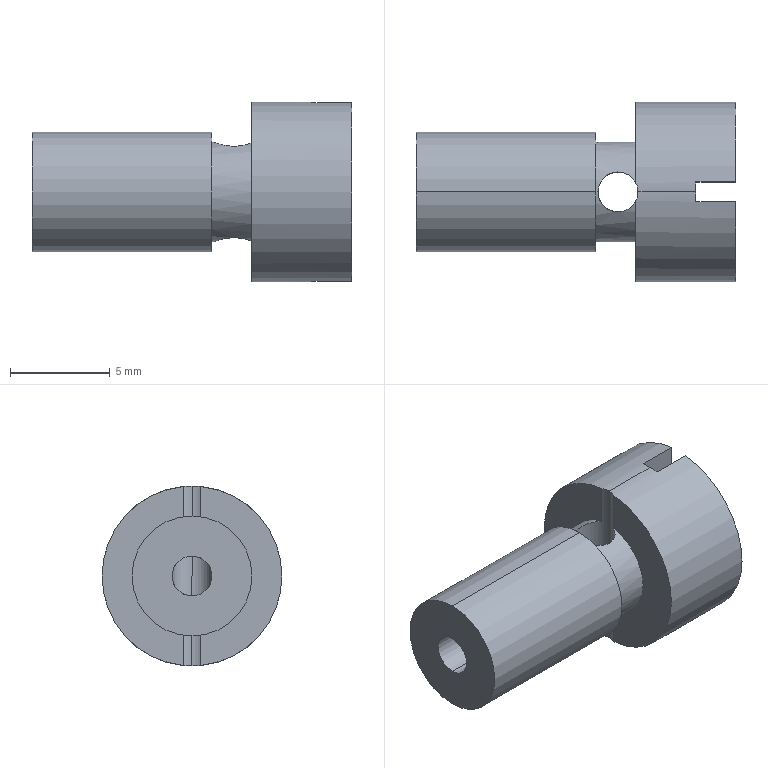Part | SolidWorks | features ICE 5, Extrusion 1 | 1 solid | 19 faces | box 16 x 9 x 9 mm | volume 549.177 mm3 | cylinder 10 | plane 9 | commonest cylinder face diameters 2 x4 5 x2 6 x2 9 x2
STEP:
#1=CARTESIAN_POINT('',(9.1,0.,-2.5));
#2=VERTEX_POINT('',#1);
#3=CARTESIAN_POINT('',(11.,-0.4359,-2.462));
#4=VERTEX_POINT('',#3);
#5=CARTESIAN_POINT('',(9.1,0.,-2.5));
#6=CARTESIAN_POINT('',(9.1,-0.1141,-2.5));
#7=CARTESIAN_POINT('',(9.119,-0.2264,-2.492));
#8=CARTESIAN_POINT('',(9.195,-0.4393,-2.463));
#9=CARTESIAN_POINT('',(9.25,-0.538,-2.443));
#10=CARTESIAN_POINT('',(9.458,-0.7984,-2.376));
#11=CARTESIAN_POINT('',(9.655,-0.9237,-2.324));
#12=CARTESIAN_POINT('',(9.985,-0.9998,-2.292));
#13=CARTESIAN_POINT('',(10.1,-1.006,-2.289));
#14=CARTESIAN_POINT('',(10.325,-0.9809,-2.3));
#15=CARTESIAN_POINT('',(10.435,-0.9488,-2.314));
#16=CARTESIAN_POINT('',(10.737,-0.8027,-2.37));
#17=CARTESIAN_POINT('',(10.901,-0.6393,-2.426));
#18=CARTESIAN_POINT('',(11.,-0.4359,-2.462));
#19=B_SPLINE_CURVE_WITH_KNOTS('',3,(#5,#6,#7,#8,#9,#10,#11,#12,#13,#14,#15,#16,#17,#18),.UNSPECIFIED.,.F.,.F.,(4,2,2,2,2,2,4),(0.002708,0.003047,0.003385,0.004061,0.004399,0.004738,0.005414),.UNSPECIFIED.);
#20=EDGE_CURVE('',#2,#4,#19,.T.);
#21=ORIENTED_EDGE('',*,*,#20,.F.);
#22=CARTESIAN_POINT('',(9.1,0.,-1.));
#23=VERTEX_POINT('',#22);
#24=CARTESIAN_POINT('',(9.1,0.,-4.5));
#25=DIRECTION('',(0.,0.,1.));
#26=VECTOR('',#25,1000.);
#27=LINE('',#24,#26);
#28=EDGE_CURVE('',#2,#23,#27,.T.);
#29=ORIENTED_EDGE('',*,*,#28,.T.);
#30=CARTESIAN_POINT('',(10.1,-1.,0.));
#31=VERTEX_POINT('',#30);
#32=CARTESIAN_POINT('',(9.1,0.,-1.));
#33=CARTESIAN_POINT('',(9.1,-0.5858,-1.));
#34=CARTESIAN_POINT('',(9.514,-1.,-0.5858));
#35=CARTESIAN_POINT('',(10.1,-1.,0.));
#36=(BOUNDED_CURVE()B_SPLINE_CURVE(3,(#32,#33,#34,#35),.UNSPECIFIED.,.F.,.T.)B_SPLINE_CURVE_WITH_KNOTS((4,4),(3.142,4.712),.UNSPECIFIED.)CURVE()GEOMETRIC_REPRESENTATION_ITEM()RATIONAL_B_SPLINE_CURVE((1.,0.8047,0.8047,1.))REPRESENTATION_ITEM(''));
#37=EDGE_CURVE('',#23,#31,#36,.T.);
#38=ORIENTED_EDGE('',*,*,#37,.T.);
#39=CARTESIAN_POINT('',(9.1,0.,1.));
#40=VERTEX_POINT('',#39);
#41=CARTESIAN_POINT('',(10.1,-1.,0.));
#42=CARTESIAN_POINT('',(9.514,-1.,0.5858));
#43=CARTESIAN_POINT('',(9.1,-0.5858,1.));
#44=CARTESIAN_POINT('',(9.1,0.,1.));
#45=(BOUNDED_CURVE()B_SPLINE_CURVE(3,(#41,#42,#43,#44),.UNSPECIFIED.,.F.,.F.)B_SPLINE_CURVE_WITH_KNOTS((4,4),(1.571,3.142),.UNSPECIFIED.)CURVE()GEOMETRIC_REPRESENTATION_ITEM()RATIONAL_B_SPLINE_CURVE((1.,0.8047,0.8047,1.))REPRESENTATION_ITEM(''));
#46=EDGE_CURVE('',#31,#40,#45,.T.);
#47=ORIENTED_EDGE('',*,*,#46,.T.);
#48=CARTESIAN_POINT('',(9.1,0.,2.5));
#49=VERTEX_POINT('',#48);
#50=CARTESIAN_POINT('',(9.1,0.,-4.5));
#51=DIRECTION('',(0.,0.,1.));
#52=VECTOR('',#51,1000.);
#53=LINE('',#50,#52);
#54=EDGE_CURVE('',#40,#49,#53,.T.);
#55=ORIENTED_EDGE('',*,*,#54,.T.);
#56=CARTESIAN_POINT('',(11.,-0.4359,2.462));
#57=VERTEX_POINT('',#56);
#58=CARTESIAN_POINT('',(11.,-0.4359,2.462));
#59=CARTESIAN_POINT('',(10.901,-0.6395,2.426));
#60=CARTESIAN_POINT('',(10.739,-0.8012,2.37));
#61=CARTESIAN_POINT('',(10.435,-0.9488,2.314));
#62=CARTESIAN_POINT('',(10.328,-0.9804,2.3));
#63=CARTESIAN_POINT('',(10.101,-1.006,2.288));
#64=CARTESIAN_POINT('',(9.987,-1.,2.291));
#65=CARTESIAN_POINT('',(9.654,-0.9237,2.324));
#66=CARTESIAN_POINT('',(9.458,-0.7988,2.376));
#67=CARTESIAN_POINT('',(9.179,-0.45,2.466));
#68=CARTESIAN_POINT('',(9.1,-0.2283,2.5));
#69=CARTESIAN_POINT('',(9.1,0.,2.5));
#70=B_SPLINE_CURVE_WITH_KNOTS('',3,(#58,#59,#60,#61,#62,#63,#64,#65,#66,#67,#68,#69),.UNSPECIFIED.,.F.,.F.,(4,2,2,2,2,4),(0.,0.0006771,0.001016,0.001354,0.002031,0.002708),.UNSPECIFIED.);
#71=EDGE_CURVE('',#57,#49,#70,.T.);
#72=ORIENTED_EDGE('',*,*,#71,.F.);
#73=CARTESIAN_POINT('',(11.,-0.4359,4.479));
#74=VERTEX_POINT('',#73);
#75=CARTESIAN_POINT('',(11.,-0.4359,-4.5));
#76=DIRECTION('',(0.,0.,-1.));
#77=VECTOR('',#76,1000.);
#78=LINE('',#75,#77);
#79=EDGE_CURVE('',#74,#57,#78,.T.);
#80=ORIENTED_EDGE('',*,*,#79,.F.);
#81=CARTESIAN_POINT('',(11.1,0.,4.5));
#82=VERTEX_POINT('',#81);
#83=CARTESIAN_POINT('',(11.1,0.,4.5));
#84=CARTESIAN_POINT('',(11.1,-0.1517,4.5));
#85=CARTESIAN_POINT('',(11.066,-0.2999,4.492));
#86=CARTESIAN_POINT('',(11.,-0.4359,4.479));
#87=B_SPLINE_CURVE_WITH_KNOTS('',3,(#83,#84,#85,#86),.UNSPECIFIED.,.F.,.F.,(4,4),(0.0004486,0.0008971),.UNSPECIFIED.);
#88=EDGE_CURVE('',#82,#74,#87,.T.);
#89=ORIENTED_EDGE('',*,*,#88,.F.);
#90=CARTESIAN_POINT('',(11.1,0.,-4.5));
#91=VERTEX_POINT('',#90);
#92=CARTESIAN_POINT('',(11.1,0.,-4.5));
#93=DIRECTION('',(0.,0.,1.));
#94=VECTOR('',#93,1000.);
#95=LINE('',#92,#94);
#96=EDGE_CURVE('',#91,#82,#95,.T.);
#97=ORIENTED_EDGE('',*,*,#96,.F.);
#98=CARTESIAN_POINT('',(11.,-0.4359,-4.479));
#99=VERTEX_POINT('',#98);
#100=CARTESIAN_POINT('',(11.,-0.4359,-4.479));
#101=CARTESIAN_POINT('',(11.066,-0.2999,-4.492));
#102=CARTESIAN_POINT('',(11.1,-0.1517,-4.5));
#103=CARTESIAN_POINT('',(11.1,0.,-4.5));
#104=B_SPLINE_CURVE_WITH_KNOTS('',3,(#100,#101,#102,#103),.UNSPECIFIED.,.F.,.F.,(4,4),(0.,0.0004486),.UNSPECIFIED.);
#105=EDGE_CURVE('',#99,#91,#104,.T.);
#106=ORIENTED_EDGE('',*,*,#105,.F.);
#107=CARTESIAN_POINT('',(11.,-0.4359,-4.5));
#108=DIRECTION('',(0.,0.,-1.));
#109=VECTOR('',#108,1000.);
#110=LINE('',#107,#109);
#111=EDGE_CURVE('',#4,#99,#110,.T.);
#112=ORIENTED_EDGE('',*,*,#111,.F.);
#113=EDGE_LOOP('',(#21,#29,#38,#47,#55,#72,#80,#89,#97,#106,#112));
#114=FACE_OUTER_BOUND('',#113,.T.);
#115=CARTESIAN_POINT('',(10.1,0.,-4.5));
#116=DIRECTION('',(0.,0.,1.));
#117=DIRECTION('',(1.,0.,0.));
#118=AXIS2_PLACEMENT_3D('',#115,#116,#117);
#119=CYLINDRICAL_SURFACE('',#118,1.);
#120=ADVANCED_FACE('',(#114),#119,.F.);
#121=CARTESIAN_POINT('',(0.,0.,-1.));
#122=VERTEX_POINT('',#121);
#123=CARTESIAN_POINT('',(0.,0.,1.));
#124=VERTEX_POINT('',#123);
#125=CARTESIAN_POINT('',(0.,0.,0.));
#126=DIRECTION('',(-1.,0.,0.));
#127=DIRECTION('',(0.,0.,-1.));
#128=AXIS2_PLACEMENT_3D('',#125,#126,#127);
#129=CIRCLE('',#128,1.);
#130=EDGE_CURVE('',#122,#124,#129,.T.);
#131=ORIENTED_EDGE('',*,*,#130,.T.);
#132=CARTESIAN_POINT('',(-0.000012,0.,1.));
#133=DIRECTION('',(1.,0.,0.));
#134=VECTOR('',#133,1000.);
#135=LINE('',#132,#134);
#136=EDGE_CURVE('',#124,#40,#135,.T.);
#137=ORIENTED_EDGE('',*,*,#136,.T.);
#138=ORIENTED_EDGE('',*,*,#46,.F.);
#139=ORIENTED_EDGE('',*,*,#37,.F.);
#140=CARTESIAN_POINT('',(-0.000012,0.,-1.));
#141=DIRECTION('',(1.,0.,0.));
#142=VECTOR('',#141,1000.);
#143=LINE('',#140,#142);
#144=EDGE_CURVE('',#122,#23,#143,.T.);
#145=ORIENTED_EDGE('',*,*,#144,.F.);
#146=EDGE_LOOP('',(#131,#137,#138,#139,#145));
#147=FACE_OUTER_BOUND('',#146,.T.);
#148=CARTESIAN_POINT('',(-0.000012,0.,0.));
#149=DIRECTION('',(1.,0.,0.));
#150=DIRECTION('',(0.,0.,-1.));
#151=AXIS2_PLACEMENT_3D('',#148,#149,#150);
#152=CYLINDRICAL_SURFACE('',#151,1.);
#153=ADVANCED_FACE('',(#147),#152,.F.);
#154=CARTESIAN_POINT('',(14.,0.5,-4.472));
#155=VERTEX_POINT('',#154);
#156=CARTESIAN_POINT('',(14.,0.,-4.5));
#157=VERTEX_POINT('',#156);
#158=CARTESIAN_POINT('',(14.,0.,0.));
#159=DIRECTION('',(-1.,0.,0.));
#160=DIRECTION('',(0.,-1.,0.));
#161=AXIS2_PLACEMENT_3D('',#158,#159,#160);
#162=CIRCLE('',#161,4.5);
#163=EDGE_CURVE('',#155,#157,#162,.T.);
#164=ORIENTED_EDGE('',*,*,#163,.T.);
#165=CARTESIAN_POINT('',(16.,0.,-4.5));
#166=DIRECTION('',(-1.,0.,0.));
#167=VECTOR('',#166,1000.);
#168=LINE('',#165,#167);
#169=EDGE_CURVE('',#157,#91,#168,.T.);
#170=ORIENTED_EDGE('',*,*,#169,.T.);
#171=CARTESIAN_POINT('',(11.,0.4359,-4.479));
#172=VERTEX_POINT('',#171);
#173=CARTESIAN_POINT('',(11.1,0.,-4.5));
#174=CARTESIAN_POINT('',(11.1,0.1517,-4.5));
#175=CARTESIAN_POINT('',(11.066,0.2999,-4.492));
#176=CARTESIAN_POINT('',(11.,0.4359,-4.479));
#177=B_SPLINE_CURVE_WITH_KNOTS('',3,(#173,#174,#175,#176),.UNSPECIFIED.,.F.,.F.,(4,4),(0.0004486,0.0008971),.UNSPECIFIED.);
#178=EDGE_CURVE('',#91,#172,#177,.T.);
#179=ORIENTED_EDGE('',*,*,#178,.T.);
#180=CARTESIAN_POINT('',(11.,0.4359,4.479));
#181=VERTEX_POINT('',#180);
#182=CARTESIAN_POINT('',(11.,0.,0.));
#183=DIRECTION('',(1.,0.,0.));
#184=DIRECTION('',(0.,0.,-1.));
#185=AXIS2_PLACEMENT_3D('',#182,#183,#184);
#186=CIRCLE('',#185,4.5);
#187=EDGE_CURVE('',#172,#181,#186,.T.);
#188=ORIENTED_EDGE('',*,*,#187,.T.);
#189=CARTESIAN_POINT('',(11.,0.4359,4.479));
#190=CARTESIAN_POINT('',(11.066,0.2999,4.492));
#191=CARTESIAN_POINT('',(11.1,0.1517,4.5));
#192=CARTESIAN_POINT('',(11.1,0.,4.5));
#193=B_SPLINE_CURVE_WITH_KNOTS('',3,(#189,#190,#191,#192),.UNSPECIFIED.,.F.,.F.,(4,4),(0.,0.0004486),.UNSPECIFIED.);
#194=EDGE_CURVE('',#181,#82,#193,.T.);
#195=ORIENTED_EDGE('',*,*,#194,.T.);
#196=CARTESIAN_POINT('',(14.,0.,4.5));
#197=VERTEX_POINT('',#196);
#198=CARTESIAN_POINT('',(16.,0.,4.5));
#199=DIRECTION('',(-1.,0.,0.));
#200=VECTOR('',#199,1000.);
#201=LINE('',#198,#200);
#202=EDGE_CURVE('',#197,#82,#201,.T.);
#203=ORIENTED_EDGE('',*,*,#202,.F.);
#204=CARTESIAN_POINT('',(14.,0.5,4.472));
#205=VERTEX_POINT('',#204);
#206=CARTESIAN_POINT('',(14.,0.,0.));
#207=DIRECTION('',(-1.,0.,0.));
#208=DIRECTION('',(0.,-1.,0.));
#209=AXIS2_PLACEMENT_3D('',#206,#207,#208);
#210=CIRCLE('',#209,4.5);
#211=EDGE_CURVE('',#197,#205,#210,.T.);
#212=ORIENTED_EDGE('',*,*,#211,.T.);
#213=CARTESIAN_POINT('',(16.,0.5,4.472));
#214=VERTEX_POINT('',#213);
#215=CARTESIAN_POINT('',(16.,0.5,4.472));
#216=DIRECTION('',(1.,0.,0.));
#217=VECTOR('',#216,1000.);
#218=LINE('',#215,#217);
#219=EDGE_CURVE('',#205,#214,#218,.T.);
#220=ORIENTED_EDGE('',*,*,#219,.T.);
#221=CARTESIAN_POINT('',(16.,0.5,-4.472));
#222=VERTEX_POINT('',#221);
#223=CARTESIAN_POINT('',(16.,0.,0.));
#224=DIRECTION('',(1.,0.,0.));
#225=DIRECTION('',(0.,0.,-1.));
#226=AXIS2_PLACEMENT_3D('',#223,#224,#225);
#227=CIRCLE('',#226,4.5);
#228=EDGE_CURVE('',#222,#214,#227,.T.);
#229=ORIENTED_EDGE('',*,*,#228,.F.);
#230=CARTESIAN_POINT('',(16.,0.5,-4.472));
#231=DIRECTION('',(-1.,0.,0.));
#232=VECTOR('',#231,1000.);
#233=LINE('',#230,#232);
#234=EDGE_CURVE('',#222,#155,#233,.T.);
#235=ORIENTED_EDGE('',*,*,#234,.T.);
#236=EDGE_LOOP('',(#164,#170,#179,#188,#195,#203,#212,#220,#229,#235));
#237=FACE_OUTER_BOUND('',#236,.T.);
#238=CARTESIAN_POINT('',(16.,0.,0.));
#239=DIRECTION('',(-1.,0.,0.));
#240=DIRECTION('',(0.,0.,1.));
#241=AXIS2_PLACEMENT_3D('',#238,#239,#240);
#242=CYLINDRICAL_SURFACE('',#241,4.5);
#243=ADVANCED_FACE('',(#237),#242,.T.);
#244=CARTESIAN_POINT('',(11.,0.4359,-2.462));
#245=VERTEX_POINT('',#244);
#246=CARTESIAN_POINT('',(11.,0.4359,-2.462));
#247=CARTESIAN_POINT('',(10.901,0.6395,-2.426));
#248=CARTESIAN_POINT('',(10.739,0.8012,-2.37));
#249=CARTESIAN_POINT('',(10.435,0.9488,-2.314));
#250=CARTESIAN_POINT('',(10.328,0.9804,-2.3));
#251=CARTESIAN_POINT('',(10.101,1.006,-2.288));
#252=CARTESIAN_POINT('',(9.987,1.,-2.291));
#253=CARTESIAN_POINT('',(9.654,0.9237,-2.324));
#254=CARTESIAN_POINT('',(9.458,0.7988,-2.376));
#255=CARTESIAN_POINT('',(9.179,0.45,-2.466));
#256=CARTESIAN_POINT('',(9.1,0.2283,-2.5));
#257=CARTESIAN_POINT('',(9.1,0.,-2.5));
#258=B_SPLINE_CURVE_WITH_KNOTS('',3,(#246,#247,#248,#249,#250,#251,#252,#253,#254,#255,#256,#257),.UNSPECIFIED.,.F.,.F.,(4,2,2,2,2,4),(0.,0.0006771,0.001016,0.001354,0.002031,0.002708),.UNSPECIFIED.);
#259=EDGE_CURVE('',#245,#2,#258,.T.);
#260=ORIENTED_EDGE('',*,*,#259,.T.);
#261=CARTESIAN_POINT('',(9.,0.,-2.5));
#262=VERTEX_POINT('',#261);
#263=CARTESIAN_POINT('',(11.,0.,-2.5));
#264=DIRECTION('',(-1.,0.,0.));
#265=VECTOR('',#264,1000.);
#266=LINE('',#263,#265);
#267=EDGE_CURVE('',#2,#262,#266,.T.);
#268=ORIENTED_EDGE('',*,*,#267,.T.);
#269=CARTESIAN_POINT('',(9.,0.,2.5));
#270=VERTEX_POINT('',#269);
#271=CARTESIAN_POINT('',(9.,0.,0.));
#272=DIRECTION('',(1.,0.,0.));
#273=DIRECTION('',(0.,0.,-1.));
#274=AXIS2_PLACEMENT_3D('',#271,#272,#273);
#275=CIRCLE('',#274,2.5);
#276=EDGE_CURVE('',#262,#270,#275,.T.);
#277=ORIENTED_EDGE('',*,*,#276,.T.);
#278=CARTESIAN_POINT('',(11.,0.,2.5));
#279=DIRECTION('',(-1.,0.,0.));
#280=VECTOR('',#279,1000.);
#281=LINE('',#278,#280);
#282=EDGE_CURVE('',#49,#270,#281,.T.);
#283=ORIENTED_EDGE('',*,*,#282,.F.);
#284=CARTESIAN_POINT('',(11.,0.4359,2.462));
#285=VERTEX_POINT('',#284);
#286=CARTESIAN_POINT('',(9.1,0.,2.5));
#287=CARTESIAN_POINT('',(9.1,0.1141,2.5));
#288=CARTESIAN_POINT('',(9.119,0.2264,2.492));
#289=CARTESIAN_POINT('',(9.195,0.4393,2.463));
#290=CARTESIAN_POINT('',(9.25,0.538,2.443));
#291=CARTESIAN_POINT('',(9.458,0.7984,2.376));
#292=CARTESIAN_POINT('',(9.655,0.9237,2.324));
#293=CARTESIAN_POINT('',(9.985,0.9998,2.292));
#294=CARTESIAN_POINT('',(10.1,1.006,2.289));
#295=CARTESIAN_POINT('',(10.325,0.9809,2.3));
#296=CARTESIAN_POINT('',(10.435,0.9488,2.314));
#297=CARTESIAN_POINT('',(10.737,0.8027,2.37));
#298=CARTESIAN_POINT('',(10.901,0.6393,2.426));
#299=CARTESIAN_POINT('',(11.,0.4359,2.462));
#300=B_SPLINE_CURVE_WITH_KNOTS('',3,(#286,#287,#288,#289,#290,#291,#292,#293,#294,#295,#296,#297,#298,#299),.UNSPECIFIED.,.F.,.F.,(4,2,2,2,2,2,4),(0.002708,0.003047,0.003385,0.004061,0.004399,0.004738,0.005414),.UNSPECIFIED.);
#301=EDGE_CURVE('',#49,#285,#300,.T.);
#302=ORIENTED_EDGE('',*,*,#301,.T.);
#303=CARTESIAN_POINT('',(11.,0.,0.));
#304=DIRECTION('',(1.,0.,0.));
#305=DIRECTION('',(0.,0.,-1.));
#306=AXIS2_PLACEMENT_3D('',#303,#304,#305);
#307=CIRCLE('',#306,2.5);
#308=EDGE_CURVE('',#245,#285,#307,.T.);
#309=ORIENTED_EDGE('',*,*,#308,.F.);
#310=EDGE_LOOP('',(#260,#268,#277,#283,#302,#309));
#311=FACE_OUTER_BOUND('',#310,.T.);
#312=CARTESIAN_POINT('',(11.,0.,0.));
#313=DIRECTION('',(-1.,0.,0.));
#314=DIRECTION('',(0.,0.,1.));
#315=AXIS2_PLACEMENT_3D('',#312,#313,#314);
#316=CYLINDRICAL_SURFACE('',#315,2.5);
#317=ADVANCED_FACE('',(#311),#316,.T.);
#318=CARTESIAN_POINT('',(9.,0.,-3.));
#319=VERTEX_POINT('',#318);
#320=CARTESIAN_POINT('',(9.,0.,3.));
#321=VERTEX_POINT('',#320);
#322=CARTESIAN_POINT('',(9.,0.,0.));
#323=DIRECTION('',(1.,0.,0.));
#324=DIRECTION('',(0.,0.,-1.));
#325=AXIS2_PLACEMENT_3D('',#322,#323,#324);
#326=CIRCLE('',#325,3.);
#327=EDGE_CURVE('',#319,#321,#326,.T.);
#328=ORIENTED_EDGE('',*,*,#327,.F.);
#329=CARTESIAN_POINT('',(0.,0.,-3.));
#330=VERTEX_POINT('',#329);
#331=CARTESIAN_POINT('',(9.,0.,-3.));
#332=DIRECTION('',(-1.,0.,0.));
#333=VECTOR('',#332,1000.);
#334=LINE('',#331,#333);
#335=EDGE_CURVE('',#319,#330,#334,.T.);
#336=ORIENTED_EDGE('',*,*,#335,.T.);
#337=CARTESIAN_POINT('',(0.,0.,3.));
#338=VERTEX_POINT('',#337);
#339=CARTESIAN_POINT('',(0.,0.,0.));
#340=DIRECTION('',(1.,0.,0.));
#341=DIRECTION('',(0.,0.,-1.));
#342=AXIS2_PLACEMENT_3D('',#339,#340,#341);
#343=CIRCLE('',#342,3.);
#344=EDGE_CURVE('',#330,#338,#343,.T.);
#345=ORIENTED_EDGE('',*,*,#344,.T.);
#346=CARTESIAN_POINT('',(9.,0.,3.));
#347=DIRECTION('',(-1.,0.,0.));
#348=VECTOR('',#347,1000.);
#349=LINE('',#346,#348);
#350=EDGE_CURVE('',#321,#338,#349,.T.);
#351=ORIENTED_EDGE('',*,*,#350,.F.);
#352=EDGE_LOOP('',(#328,#336,#345,#351));
#353=FACE_OUTER_BOUND('',#352,.T.);
#354=CARTESIAN_POINT('',(9.,0.,0.));
#355=DIRECTION('',(-1.,0.,0.));
#356=DIRECTION('',(0.,0.,1.));
#357=AXIS2_PLACEMENT_3D('',#354,#355,#356);
#358=CYLINDRICAL_SURFACE('',#357,3.);
#359=ADVANCED_FACE('',(#353),#358,.T.);
#360=CARTESIAN_POINT('',(16.,-0.5,4.472));
#361=VERTEX_POINT('',#360);
#362=CARTESIAN_POINT('',(16.,-0.5,-4.472));
#363=VERTEX_POINT('',#362);
#364=CARTESIAN_POINT('',(16.,-0.5,0.));
#365=DIRECTION('',(0.,0.,-1.));
#366=VECTOR('',#365,1000.);
#367=LINE('',#364,#366);
#368=EDGE_CURVE('',#361,#363,#367,.T.);
#369=ORIENTED_EDGE('',*,*,#368,.F.);
#370=CARTESIAN_POINT('',(16.,0.,0.));
#371=DIRECTION('',(1.,0.,0.));
#372=DIRECTION('',(0.,0.,-1.));
#373=AXIS2_PLACEMENT_3D('',#370,#371,#372);
#374=CIRCLE('',#373,4.5);
#375=EDGE_CURVE('',#361,#363,#374,.T.);
#376=ORIENTED_EDGE('',*,*,#375,.T.);
#377=EDGE_LOOP('',(#369,#376));
#378=FACE_OUTER_BOUND('',#377,.T.);
#379=CARTESIAN_POINT('',(16.,0.,0.));
#380=DIRECTION('',(1.,0.,0.));
#381=DIRECTION('',(0.,0.,-1.));
#382=AXIS2_PLACEMENT_3D('',#379,#380,#381);
#383=PLANE('',#382);
#384=ADVANCED_FACE('',(#378),#383,.T.);
#385=ORIENTED_EDGE('',*,*,#187,.F.);
#386=CARTESIAN_POINT('',(11.,0.4359,-4.5));
#387=DIRECTION('',(0.,0.,1.));
#388=VECTOR('',#387,1000.);
#389=LINE('',#386,#388);
#390=EDGE_CURVE('',#172,#245,#389,.T.);
#391=ORIENTED_EDGE('',*,*,#390,.T.);
#392=ORIENTED_EDGE('',*,*,#308,.T.);
#393=CARTESIAN_POINT('',(11.,0.4359,-4.5));
#394=DIRECTION('',(0.,0.,1.));
#395=VECTOR('',#394,1000.);
#396=LINE('',#393,#395);
#397=EDGE_CURVE('',#285,#181,#396,.T.);
#398=ORIENTED_EDGE('',*,*,#397,.T.);
#399=EDGE_LOOP('',(#385,#391,#392,#398));
#400=FACE_OUTER_BOUND('',#399,.T.);
#401=CARTESIAN_POINT('',(11.,0.,0.));
#402=DIRECTION('',(1.,0.,0.));
#403=DIRECTION('',(0.,0.,-1.));
#404=AXIS2_PLACEMENT_3D('',#401,#402,#403);
#405=PLANE('',#404);
#406=ADVANCED_FACE('',(#400),#405,.F.);
#407=ORIENTED_EDGE('',*,*,#335,.F.);
#408=CARTESIAN_POINT('',(9.,0.,0.));
#409=DIRECTION('',(1.,0.,0.));
#410=DIRECTION('',(0.,0.,-1.));
#411=AXIS2_PLACEMENT_3D('',#408,#409,#410);
#412=CIRCLE('',#411,3.);
#413=EDGE_CURVE('',#321,#319,#412,.T.);
#414=ORIENTED_EDGE('',*,*,#413,.F.);
#415=ORIENTED_EDGE('',*,*,#350,.T.);
#416=CARTESIAN_POINT('',(0.,0.,0.));
#417=DIRECTION('',(1.,0.,0.));
#418=DIRECTION('',(0.,0.,-1.));
#419=AXIS2_PLACEMENT_3D('',#416,#417,#418);
#420=CIRCLE('',#419,3.);
#421=EDGE_CURVE('',#338,#330,#420,.T.);
#422=ORIENTED_EDGE('',*,*,#421,.T.);
#423=EDGE_LOOP('',(#407,#414,#415,#422));
#424=FACE_OUTER_BOUND('',#423,.T.);
#425=CARTESIAN_POINT('',(9.,0.,0.));
#426=DIRECTION('',(-1.,0.,0.));
#427=DIRECTION('',(0.,0.,1.));
#428=AXIS2_PLACEMENT_3D('',#425,#426,#427);
#429=CYLINDRICAL_SURFACE('',#428,3.);
#430=ADVANCED_FACE('',(#424),#429,.T.);
#431=CARTESIAN_POINT('',(9.,0.,0.));
#432=DIRECTION('',(1.,0.,0.));
#433=DIRECTION('',(0.,0.,-1.));
#434=AXIS2_PLACEMENT_3D('',#431,#432,#433);
#435=CIRCLE('',#434,2.5);
#436=EDGE_CURVE('',#270,#262,#435,.T.);
#437=ORIENTED_EDGE('',*,*,#436,.F.);
#438=ORIENTED_EDGE('',*,*,#276,.F.);
#439=EDGE_LOOP('',(#437,#438));
#440=FACE_BOUND('',#439,.T.);
#441=ORIENTED_EDGE('',*,*,#413,.T.);
#442=ORIENTED_EDGE('',*,*,#327,.T.);
#443=EDGE_LOOP('',(#441,#442));
#444=FACE_OUTER_BOUND('',#443,.T.);
#445=CARTESIAN_POINT('',(9.,0.,0.));
#446=DIRECTION('',(1.,0.,0.));
#447=DIRECTION('',(0.,0.,-1.));
#448=AXIS2_PLACEMENT_3D('',#445,#446,#447);
#449=PLANE('',#448);
#450=ADVANCED_FACE('',(#440,#444),#449,.T.);
#451=ORIENTED_EDGE('',*,*,#130,.F.);
#452=CARTESIAN_POINT('',(0.,0.,0.));
#453=DIRECTION('',(-1.,0.,0.));
#454=DIRECTION('',(0.,0.,-1.));
#455=AXIS2_PLACEMENT_3D('',#452,#453,#454);
#456=CIRCLE('',#455,1.);
#457=EDGE_CURVE('',#124,#122,#456,.T.);
#458=ORIENTED_EDGE('',*,*,#457,.F.);
#459=EDGE_LOOP('',(#451,#458));
#460=FACE_BOUND('',#459,.T.);
#461=ORIENTED_EDGE('',*,*,#421,.F.);
#462=ORIENTED_EDGE('',*,*,#344,.F.);
#463=EDGE_LOOP('',(#461,#462));
#464=FACE_OUTER_BOUND('',#463,.T.);
#465=CARTESIAN_POINT('',(0.,0.,0.));
#466=DIRECTION('',(1.,0.,0.));
#467=DIRECTION('',(0.,0.,-1.));
#468=AXIS2_PLACEMENT_3D('',#465,#466,#467);
#469=PLANE('',#468);
#470=ADVANCED_FACE('',(#460,#464),#469,.F.);
#471=ORIENTED_EDGE('',*,*,#267,.F.);
#472=ORIENTED_EDGE('',*,*,#20,.T.);
#473=CARTESIAN_POINT('',(11.,0.,0.));
#474=DIRECTION('',(1.,0.,0.));
#475=DIRECTION('',(0.,0.,-1.));
#476=AXIS2_PLACEMENT_3D('',#473,#474,#475);
#477=CIRCLE('',#476,2.5);
#478=EDGE_CURVE('',#57,#4,#477,.T.);
#479=ORIENTED_EDGE('',*,*,#478,.F.);
#480=ORIENTED_EDGE('',*,*,#71,.T.);
#481=ORIENTED_EDGE('',*,*,#282,.T.);
#482=ORIENTED_EDGE('',*,*,#436,.T.);
#483=EDGE_LOOP('',(#471,#472,#479,#480,#481,#482));
#484=FACE_OUTER_BOUND('',#483,.T.);
#485=CARTESIAN_POINT('',(11.,0.,0.));
#486=DIRECTION('',(-1.,0.,0.));
#487=DIRECTION('',(0.,0.,1.));
#488=AXIS2_PLACEMENT_3D('',#485,#486,#487);
#489=CYLINDRICAL_SURFACE('',#488,2.5);
#490=ADVANCED_FACE('',(#484),#489,.T.);
#491=ORIENTED_EDGE('',*,*,#169,.F.);
#492=CARTESIAN_POINT('',(14.,-0.5,-4.472));
#493=VERTEX_POINT('',#492);
#494=CARTESIAN_POINT('',(14.,0.,0.));
#495=DIRECTION('',(-1.,0.,0.));
#496=DIRECTION('',(0.,-1.,0.));
#497=AXIS2_PLACEMENT_3D('',#494,#495,#496);
#498=CIRCLE('',#497,4.5);
#499=EDGE_CURVE('',#157,#493,#498,.T.);
#500=ORIENTED_EDGE('',*,*,#499,.T.);
#501=CARTESIAN_POINT('',(16.,-0.5,-4.472));
#502=DIRECTION('',(1.,0.,0.));
#503=VECTOR('',#502,1000.);
#504=LINE('',#501,#503);
#505=EDGE_CURVE('',#493,#363,#504,.T.);
#506=ORIENTED_EDGE('',*,*,#505,.T.);
#507=ORIENTED_EDGE('',*,*,#375,.F.);
#508=CARTESIAN_POINT('',(14.,-0.5,4.472));
#509=VERTEX_POINT('',#508);
#510=CARTESIAN_POINT('',(16.,-0.5,4.472));
#511=DIRECTION('',(-1.,0.,0.));
#512=VECTOR('',#511,1000.);
#513=LINE('',#510,#512);
#514=EDGE_CURVE('',#361,#509,#513,.T.);
#515=ORIENTED_EDGE('',*,*,#514,.T.);
#516=CARTESIAN_POINT('',(14.,0.,0.));
#517=DIRECTION('',(-1.,0.,0.));
#518=DIRECTION('',(0.,-1.,0.));
#519=AXIS2_PLACEMENT_3D('',#516,#517,#518);
#520=CIRCLE('',#519,4.5);
#521=EDGE_CURVE('',#509,#197,#520,.T.);
#522=ORIENTED_EDGE('',*,*,#521,.T.);
#523=ORIENTED_EDGE('',*,*,#202,.T.);
#524=ORIENTED_EDGE('',*,*,#88,.T.);
#525=CARTESIAN_POINT('',(11.,0.,0.));
#526=DIRECTION('',(1.,0.,0.));
#527=DIRECTION('',(0.,0.,-1.));
#528=AXIS2_PLACEMENT_3D('',#525,#526,#527);
#529=CIRCLE('',#528,4.5);
#530=EDGE_CURVE('',#74,#99,#529,.T.);
#531=ORIENTED_EDGE('',*,*,#530,.T.);
#532=ORIENTED_EDGE('',*,*,#105,.T.);
#533=EDGE_LOOP('',(#491,#500,#506,#507,#515,#522,#523,#524,#531,#532));
#534=FACE_OUTER_BOUND('',#533,.T.);
#535=CARTESIAN_POINT('',(16.,0.,0.));
#536=DIRECTION('',(-1.,0.,0.));
#537=DIRECTION('',(0.,0.,1.));
#538=AXIS2_PLACEMENT_3D('',#535,#536,#537);
#539=CYLINDRICAL_SURFACE('',#538,4.5);
#540=ADVANCED_FACE('',(#534),#539,.T.);
#541=CARTESIAN_POINT('',(16.,0.5,0.));
#542=DIRECTION('',(0.,0.,1.));
#543=VECTOR('',#542,1000.);
#544=LINE('',#541,#543);
#545=EDGE_CURVE('',#222,#214,#544,.T.);
#546=ORIENTED_EDGE('',*,*,#545,.F.);
#547=ORIENTED_EDGE('',*,*,#228,.T.);
#548=EDGE_LOOP('',(#546,#547));
#549=FACE_OUTER_BOUND('',#548,.T.);
#550=CARTESIAN_POINT('',(16.,0.,0.));
#551=DIRECTION('',(1.,0.,0.));
#552=DIRECTION('',(0.,0.,-1.));
#553=AXIS2_PLACEMENT_3D('',#550,#551,#552);
#554=PLANE('',#553);
#555=ADVANCED_FACE('',(#549),#554,.T.);
#556=ORIENTED_EDGE('',*,*,#530,.F.);
#557=ORIENTED_EDGE('',*,*,#79,.T.);
#558=ORIENTED_EDGE('',*,*,#478,.T.);
#559=ORIENTED_EDGE('',*,*,#111,.T.);
#560=EDGE_LOOP('',(#556,#557,#558,#559));
#561=FACE_OUTER_BOUND('',#560,.T.);
#562=CARTESIAN_POINT('',(11.,0.,0.));
#563=DIRECTION('',(1.,0.,0.));
#564=DIRECTION('',(0.,0.,-1.));
#565=AXIS2_PLACEMENT_3D('',#562,#563,#564);
#566=PLANE('',#565);
#567=ADVANCED_FACE('',(#561),#566,.F.);
#568=ORIENTED_EDGE('',*,*,#136,.F.);
#569=ORIENTED_EDGE('',*,*,#457,.T.);
#570=ORIENTED_EDGE('',*,*,#144,.T.);
#571=CARTESIAN_POINT('',(10.1,1.,0.));
#572=VERTEX_POINT('',#571);
#573=CARTESIAN_POINT('',(10.1,1.,0.));
#574=CARTESIAN_POINT('',(9.514,1.,-0.5858));
#575=CARTESIAN_POINT('',(9.1,0.5858,-1.));
#576=CARTESIAN_POINT('',(9.1,0.,-1.));
#577=(BOUNDED_CURVE()B_SPLINE_CURVE(3,(#573,#574,#575,#576),.UNSPECIFIED.,.F.,.T.)B_SPLINE_CURVE_WITH_KNOTS((4,4),(1.571,3.142),.UNSPECIFIED.)CURVE()GEOMETRIC_REPRESENTATION_ITEM()RATIONAL_B_SPLINE_CURVE((1.,0.8047,0.8047,1.))REPRESENTATION_ITEM(''));
#578=EDGE_CURVE('',#572,#23,#577,.T.);
#579=ORIENTED_EDGE('',*,*,#578,.F.);
#580=CARTESIAN_POINT('',(9.1,0.,1.));
#581=CARTESIAN_POINT('',(9.1,0.5858,1.));
#582=CARTESIAN_POINT('',(9.514,1.,0.5858));
#583=CARTESIAN_POINT('',(10.1,1.,0.));
#584=(BOUNDED_CURVE()B_SPLINE_CURVE(3,(#580,#581,#582,#583),.UNSPECIFIED.,.F.,.T.)B_SPLINE_CURVE_WITH_KNOTS((4,4),(3.142,4.712),.UNSPECIFIED.)CURVE()GEOMETRIC_REPRESENTATION_ITEM()RATIONAL_B_SPLINE_CURVE((1.,0.8047,0.8047,1.))REPRESENTATION_ITEM(''));
#585=EDGE_CURVE('',#40,#572,#584,.T.);
#586=ORIENTED_EDGE('',*,*,#585,.F.);
#587=EDGE_LOOP('',(#568,#569,#570,#579,#586));
#588=FACE_OUTER_BOUND('',#587,.T.);
#589=CARTESIAN_POINT('',(-0.000012,0.,0.));
#590=DIRECTION('',(1.,0.,0.));
#591=DIRECTION('',(0.,0.,-1.));
#592=AXIS2_PLACEMENT_3D('',#589,#590,#591);
#593=CYLINDRICAL_SURFACE('',#592,1.);
#594=ADVANCED_FACE('',(#588),#593,.F.);
#595=ORIENTED_EDGE('',*,*,#28,.F.);
#596=ORIENTED_EDGE('',*,*,#259,.F.);
#597=ORIENTED_EDGE('',*,*,#390,.F.);
#598=ORIENTED_EDGE('',*,*,#178,.F.);
#599=ORIENTED_EDGE('',*,*,#96,.T.);
#600=ORIENTED_EDGE('',*,*,#194,.F.);
#601=ORIENTED_EDGE('',*,*,#397,.F.);
#602=ORIENTED_EDGE('',*,*,#301,.F.);
#603=ORIENTED_EDGE('',*,*,#54,.F.);
#604=ORIENTED_EDGE('',*,*,#585,.T.);
#605=ORIENTED_EDGE('',*,*,#578,.T.);
#606=EDGE_LOOP('',(#595,#596,#597,#598,#599,#600,#601,#602,#603,#604,#605));
#607=FACE_OUTER_BOUND('',#606,.T.);
#608=CARTESIAN_POINT('',(10.1,0.,-4.5));
#609=DIRECTION('',(0.,0.,1.));
#610=DIRECTION('',(1.,0.,0.));
#611=AXIS2_PLACEMENT_3D('',#608,#609,#610);
#612=CYLINDRICAL_SURFACE('',#611,1.);
#613=ADVANCED_FACE('',(#607),#612,.F.);
#614=CARTESIAN_POINT('',(14.,-0.5,-4.5));
#615=DIRECTION('',(0.,0.,1.));
#616=VECTOR('',#615,1000.);
#617=LINE('',#614,#616);
#618=EDGE_CURVE('',#493,#509,#617,.T.);
#619=ORIENTED_EDGE('',*,*,#618,.F.);
#620=ORIENTED_EDGE('',*,*,#499,.F.);
#621=ORIENTED_EDGE('',*,*,#163,.F.);
#622=CARTESIAN_POINT('',(14.,0.5,-4.5));
#623=DIRECTION('',(0.,0.,1.));
#624=VECTOR('',#623,1000.);
#625=LINE('',#622,#624);
#626=EDGE_CURVE('',#155,#205,#625,.T.);
#627=ORIENTED_EDGE('',*,*,#626,.T.);
#628=ORIENTED_EDGE('',*,*,#211,.F.);
#629=ORIENTED_EDGE('',*,*,#521,.F.);
#630=EDGE_LOOP('',(#619,#620,#621,#627,#628,#629));
#631=FACE_OUTER_BOUND('',#630,.T.);
#632=CARTESIAN_POINT('',(14.,0.5,-4.5));
#633=DIRECTION('',(-1.,0.,0.));
#634=DIRECTION('',(0.,-1.,0.));
#635=AXIS2_PLACEMENT_3D('',#632,#633,#634);
#636=PLANE('',#635);
#637=ADVANCED_FACE('',(#631),#636,.F.);
#638=ORIENTED_EDGE('',*,*,#368,.T.);
#639=ORIENTED_EDGE('',*,*,#505,.F.);
#640=ORIENTED_EDGE('',*,*,#618,.T.);
#641=ORIENTED_EDGE('',*,*,#514,.F.);
#642=EDGE_LOOP('',(#638,#639,#640,#641));
#643=FACE_OUTER_BOUND('',#642,.T.);
#644=CARTESIAN_POINT('',(14.,-0.5,-4.5));
#645=DIRECTION('',(0.,-1.,0.));
#646=DIRECTION('',(0.,0.,-1.));
#647=AXIS2_PLACEMENT_3D('',#644,#645,#646);
#648=PLANE('',#647);
#649=ADVANCED_FACE('',(#643),#648,.F.);
#650=ORIENTED_EDGE('',*,*,#545,.T.);
#651=ORIENTED_EDGE('',*,*,#219,.F.);
#652=ORIENTED_EDGE('',*,*,#626,.F.);
#653=ORIENTED_EDGE('',*,*,#234,.F.);
#654=EDGE_LOOP('',(#650,#651,#652,#653));
#655=FACE_OUTER_BOUND('',#654,.T.);
#656=CARTESIAN_POINT('',(14.,0.5,-4.5));
#657=DIRECTION('',(0.,1.,0.));
#658=DIRECTION('',(0.,0.,1.));
#659=AXIS2_PLACEMENT_3D('',#656,#657,#658);
#660=PLANE('',#659);
#661=ADVANCED_FACE('',(#655),#660,.F.);
#662=CLOSED_SHELL('',(#120,#153,#243,#317,#359,#384,#406,#430,#450,#470,#490,#540,#555,#567,#594,#613,#637,#649,#661));
#663=MANIFOLD_SOLID_BREP('',#662);
#664=CARTESIAN_POINT('',(0.,0.,0.));
#665=DIRECTION('',(0.,0.,1.));
#666=DIRECTION('',(1.,0.,0.));
#667=AXIS2_PLACEMENT_3D('',#664,#665,#666);
#668=(LENGTH_UNIT()NAMED_UNIT(*)SI_UNIT(.MILLI.,.METRE.));
#669=UNCERTAINTY_MEASURE_WITH_UNIT(LENGTH_MEASURE(0.00001),#668,'','');
#670=(NAMED_UNIT(*)PLANE_ANGLE_UNIT()SI_UNIT($,.RADIAN.));
#671=(NAMED_UNIT(*)SI_UNIT($,.STERADIAN.)SOLID_ANGLE_UNIT());
#672=(GEOMETRIC_REPRESENTATION_CONTEXT(3)GLOBAL_UNCERTAINTY_ASSIGNED_CONTEXT((#669))GLOBAL_UNIT_ASSIGNED_CONTEXT((#668,#670,#671))REPRESENTATION_CONTEXT('',''));
#673=ADVANCED_BREP_SHAPE_REPRESENTATION('',(#663,#667),#672);